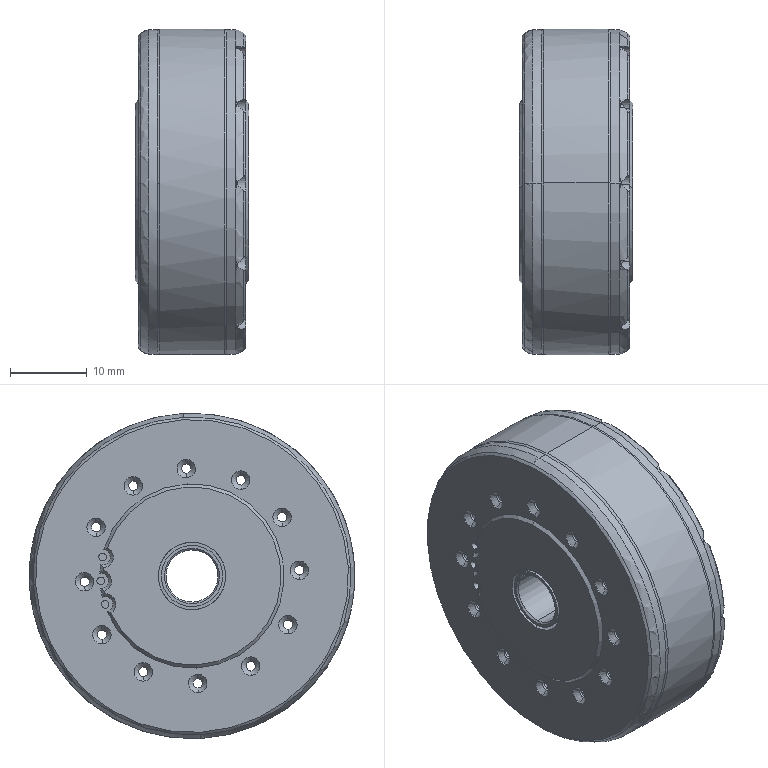Part | SolidWorks | features BaseBody 3, ICE 1, Scale 1 | 2 solids | 732 faces | box 14.8 x 42.4 x 42.4 mm | volume 8202 mm3 | cylinder 406 | plane 187 | cone 135 | spline 4 | commonest cylinder face diameters 1.2 x72 2.4 x72 33.199 x60 37.601 x32 32.8 x31 1 x30